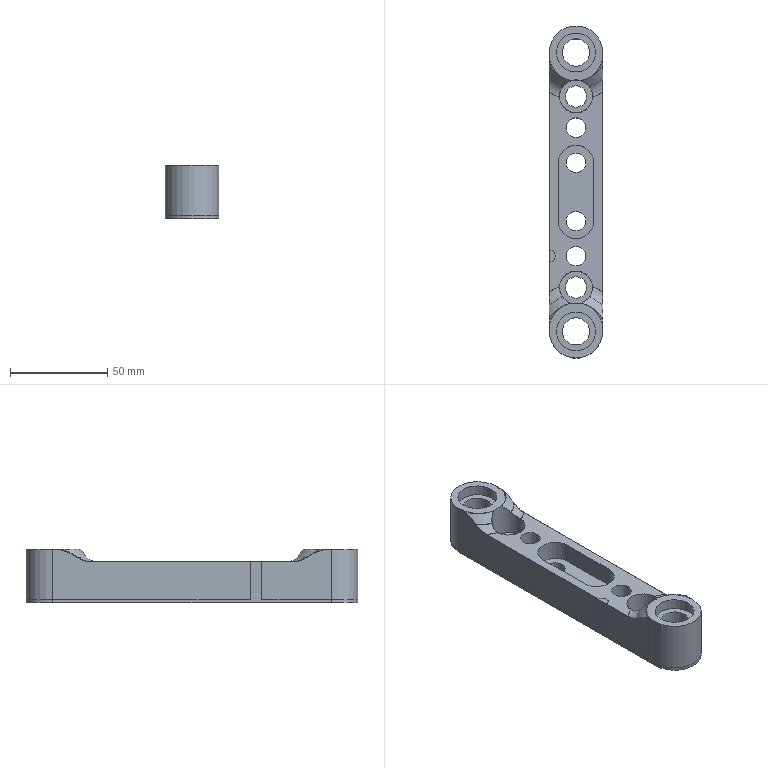NC program | NX | posted with a generic post | part box 27.4 x 170.48 x 27.5 mm
Lines 121 to 968 of 1859:
(PLANAR_MILL_12 , TOOL : D8开粗)
N204 T06 M6
N206 G54
N208 G17 G0 G90 X-73.278 Y0.754 B0. C0. S3000 M3
N210 G43 Z30. H6
N212 Z1.
N214 G94 G1 X-73.462 Y0.17 Z0.989 F600.
N216 X-73.355 Y-0.656 Z0.975
N218 X-73.016 Y-1.244 Z0.963
N220 X-72.505 Y-1.671 Z0.951
N222 X-71.879 Y-1.9 Z0.94
N224 X-71.201 Z0.928
N226 X-70.575 Y-1.671 Z0.916
N228 X-70.064 Y-1.244 Z0.905
N230 X-69.725 Y-0.656 Z0.893
N232 X-69.618 Y0.17 Z0.878
N234 X-69.869 Y0.965 Z0.864
N236 X-70.431 Y1.58 Z0.849
N238 X-71.201 Y1.9 Z0.835
N240 X-71.879 Z0.823
N242 X-72.649 Y1.58 Z0.808
N244 X-73.211 Y0.965 Z0.794
N246 X-73.462 Y0.17 Z0.779
N248 X-73.355 Y-0.656 Z0.764
N250 X-73.016 Y-1.244 Z0.753
N252 X-72.505 Y-1.671 Z0.741
N254 X-71.879 Y-1.9 Z0.729
N256 X-71.201 Z0.718
N258 X-70.575 Y-1.671 Z0.706
N260 X-70.064 Y-1.244 Z0.694
N262 X-69.725 Y-0.656 Z0.682
N264 X-69.618 Y0.17 Z0.668
N266 X-69.869 Y0.965 Z0.653
N268 X-70.431 Y1.58 Z0.639
N270 X-71.201 Y1.9 Z0.624
N272 X-71.879 Z0.612
N274 X-72.649 Y1.58 Z0.598
N276 X-73.211 Y0.965 Z0.583
N278 X-73.462 Y0.17 Z0.569
N280 X-73.355 Y-0.656 Z0.554
N282 X-73.016 Y-1.244 Z0.542
N284 X-72.505 Y-1.671 Z0.531
N286 X-71.879 Y-1.9 Z0.519
N288 X-71.201 Z0.507
N290 X-70.575 Y-1.671 Z0.496
N292 X-70.064 Y-1.244 Z0.484
N294 X-69.725 Y-0.656 Z0.472
N296 X-69.618 Y0.17 Z0.458
N298 X-69.869 Y0.965 Z0.443
N300 X-70.431 Y1.58 Z0.429
N302 X-71.201 Y1.9 Z0.414
N304 X-71.879 Z0.402
N306 X-72.649 Y1.58 Z0.388
N308 X-73.211 Y0.965 Z0.373
N310 X-73.462 Y0.17 Z0.359
N312 X-73.355 Y-0.656 Z0.344
N314 X-73.016 Y-1.244 Z0.332
N316 X-72.505 Y-1.671 Z0.321
N318 X-71.879 Y-1.9 Z0.309
N320 X-71.201 Z0.297
N322 X-70.575 Y-1.671 Z0.285
N324 X-70.064 Y-1.244 Z0.274
N326 X-69.725 Y-0.656 Z0.262
N328 X-69.618 Y0.17 Z0.247
N330 X-69.869 Y0.965 Z0.233
N332 X-70.431 Y1.58 Z0.218
N334 X-71.201 Y1.9 Z0.204
N336 X-71.879 Z0.192
N338 X-72.649 Y1.58 Z0.177
N340 X-73.211 Y0.965 Z0.163
N342 X-73.462 Y0.17 Z0.148
N344 X-73.355 Y-0.656 Z0.134
N346 X-73.016 Y-1.244 Z0.122
N348 X-72.505 Y-1.671 Z0.11
N350 X-71.879 Y-1.9 Z0.099
N352 X-71.201 Z0.087
N354 X-70.575 Y-1.671 Z0.075
N356 X-70.064 Y-1.244 Z0.064
N358 X-69.725 Y-0.656 Z0.052
N360 X-69.618 Y0.17 Z0.037
N362 X-69.869 Y0.965 Z0.023
N364 X-70.431 Y1.58 Z0.008
N366 X-71.201 Y1.9 Z-0.007
N368 X-71.879 Z-0.018
N370 X-72.649 Y1.58 Z-0.033
N372 X-73.211 Y0.965 Z-0.047
N374 X-73.462 Y0.17 Z-0.062
N376 X-73.355 Y-0.656 Z-0.077
N378 X-73.016 Y-1.244 Z-0.088
N380 X-72.505 Y-1.671 Z-0.1
N382 X-71.879 Y-1.9 Z-0.112
N384 X-71.201 Z-0.123
N386 X-70.575 Y-1.671 Z-0.135
N388 X-70.064 Y-1.244 Z-0.147
N390 X-69.725 Y-0.656 Z-0.159
N392 X-69.618 Y0.17 Z-0.173
N394 X-69.869 Y0.965 Z-0.188
N396 X-70.431 Y1.58 Z-0.202
N398 X-71.201 Y1.9 Z-0.217
N400 X-71.879 Z-0.229
N402 X-72.649 Y1.58 Z-0.243
N404 X-73.211 Y0.965 Z-0.258
N406 X-73.462 Y0.17 Z-0.272
N408 X-73.355 Y-0.656 Z-0.287
N410 X-73.016 Y-1.244 Z-0.299
N412 X-72.505 Y-1.671 Z-0.31
N414 X-71.879 Y-1.9 Z-0.322
N416 X-71.201 Z-0.334
N418 X-70.575 Y-1.671 Z-0.345
N420 X-70.064 Y-1.244 Z-0.357
N422 X-69.725 Y-0.656 Z-0.369
N424 X-69.618 Y0.17 Z-0.383
N426 X-69.869 Y0.965 Z-0.398
N428 X-70.431 Y1.58 Z-0.413
N430 X-71.201 Y1.9 Z-0.427
N432 X-71.879 Z-0.439
N434 X-72.649 Y1.58 Z-0.453
N436 X-73.211 Y0.965 Z-0.468
N438 X-73.462 Y0.17 Z-0.483
N440 X-73.355 Y-0.656 Z-0.497
N442 X-73.016 Y-1.244 Z-0.509
N444 X-72.505 Y-1.671 Z-0.521
N446 X-71.879 Y-1.9 Z-0.532
N448 X-71.201 Z-0.544
N450 X-70.575 Y-1.671 Z-0.556
N452 X-70.064 Y-1.244 Z-0.567
N454 X-69.725 Y-0.656 Z-0.579
N456 X-69.618 Y0.17 Z-0.594
N458 X-69.869 Y0.965 Z-0.608
N460 X-70.431 Y1.58 Z-0.623
N462 X-71.201 Y1.9 Z-0.637
N464 X-71.879 Z-0.649
N466 X-72.649 Y1.58 Z-0.664
N468 X-73.211 Y0.965 Z-0.678
N470 X-73.462 Y0.17 Z-0.693
N472 X-73.355 Y-0.656 Z-0.707
N474 X-73.016 Y-1.244 Z-0.719
N476 X-72.505 Y-1.671 Z-0.731
N478 X-71.879 Y-1.9 Z-0.742
N480 X-71.201 Z-0.754
N482 X-70.575 Y-1.671 Z-0.766
N484 X-70.064 Y-1.244 Z-0.778
N486 X-69.725 Y-0.656 Z-0.789
N488 X-69.618 Y0.17 Z-0.804
N490 X-69.869 Y0.965 Z-0.818
N492 X-70.431 Y1.58 Z-0.833
N494 X-71.201 Y1.9 Z-0.848
N496 X-71.879 Z-0.859
N498 X-72.649 Y1.58 Z-0.874
N500 X-73.211 Y0.965 Z-0.889
N502 X-73.462 Y0.17 Z-0.903
N504 X-73.355 Y-0.656 Z-0.918
N506 X-73.016 Y-1.244 Z-0.929
N508 X-72.505 Y-1.671 Z-0.941
N510 X-71.879 Y-1.9 Z-0.953
N512 X-71.201 Z-0.965
N514 X-70.575 Y-1.671 Z-0.976
N516 X-70.064 Y-1.244 Z-0.988
N518 X-69.725 Y-0.656 Z-1.
N520 X-69.618 Y0.17 Z-1.014
N522 X-69.869 Y0.965 Z-1.029
N524 X-70.431 Y1.58 Z-1.043
N526 X-71.201 Y1.9 Z-1.058
N528 X-71.879 Z-1.07
N530 X-72.649 Y1.58 Z-1.084
N532 X-73.211 Y0.965 Z-1.099
N534 X-73.462 Y0.17 Z-1.113
N536 X-73.355 Y-0.656 Z-1.128
N538 X-73.016 Y-1.244 Z-1.14
N540 X-72.505 Y-1.671 Z-1.151
N542 X-71.879 Y-1.9 Z-1.163
N544 X-71.201 Z-1.175
N546 X-70.575 Y-1.671 Z-1.186
N548 X-70.064 Y-1.244 Z-1.198
N550 X-69.725 Y-0.656 Z-1.21
N552 X-69.618 Y0.17 Z-1.224
N554 X-69.869 Y0.965 Z-1.239
N556 X-70.431 Y1.58 Z-1.254
N558 X-71.201 Y1.9 Z-1.268
N560 X-71.879 Z-1.28
N562 X-72.649 Y1.58 Z-1.294
N564 X-73.211 Y0.965 Z-1.309
N566 X-73.462 Y0.17 Z-1.324
N568 X-73.355 Y-0.656 Z-1.338
N570 X-73.016 Y-1.244 Z-1.35
N572 X-72.505 Y-1.671 Z-1.362
N574 X-71.879 Y-1.9 Z-1.373
N576 X-71.201 Z-1.385
N578 X-70.575 Y-1.671 Z-1.397
N580 X-70.064 Y-1.244 Z-1.408
N582 X-69.725 Y-0.656 Z-1.42
N584 X-69.618 Y0.17 Z-1.435
N586 X-69.869 Y0.965 Z-1.449
N588 X-70.431 Y1.58 Z-1.464
N590 X-71.201 Y1.9 Z-1.478
N592 X-71.879 Z-1.49
N594 X-72.649 Y1.58 Z-1.505
N596 X-73.211 Y0.965 Z-1.519
N598 X-73.462 Y0.17 Z-1.534
N600 X-73.355 Y-0.656 Z-1.548
N602 X-73.016 Y-1.244 Z-1.56
N604 X-72.505 Y-1.671 Z-1.572
N606 X-71.879 Y-1.9 Z-1.584
N608 X-71.201 Z-1.595
N610 X-70.575 Y-1.671 Z-1.607
N612 X-70.064 Y-1.244 Z-1.619
N614 X-69.725 Y-0.656 Z-1.63
N616 X-69.618 Y0.17 Z-1.645
N618 X-69.869 Y0.965 Z-1.66
N620 X-70.431 Y1.58 Z-1.674
N622 X-71.201 Y1.9 Z-1.689
N624 X-71.879 Z-1.7
N626 X-72.649 Y1.58 Z-1.715
N628 X-73.211 Y0.965 Z-1.73
N630 X-73.462 Y0.17 Z-1.744
N632 X-73.355 Y-0.656 Z-1.759
N634 X-73.016 Y-1.244 Z-1.771
N636 X-72.505 Y-1.671 Z-1.782
N638 X-71.879 Y-1.9 Z-1.794
N640 X-71.201 Z-1.806
N642 X-70.575 Y-1.671 Z-1.817
N644 X-70.064 Y-1.244 Z-1.829
N646 X-69.725 Y-0.656 Z-1.841
N648 X-69.618 Y0.17 Z-1.855
N650 X-69.869 Y0.965 Z-1.87
N652 X-70.431 Y1.58 Z-1.884
N654 X-71.201 Y1.9 Z-1.899
N656 X-71.879 Z-1.911
N658 X-72.649 Y1.58 Z-1.925
N660 X-73.211 Y0.965 Z-1.94
N662 X-73.462 Y0.17 Z-1.954
N664 X-73.355 Y-0.656 Z-1.969
N666 X-73.016 Y-1.244 Z-1.981
N668 X-72.505 Y-1.671 Z-1.992
N670 X-71.879 Y-1.9 Z-2.004
N672 X-71.201 Z-2.016
N674 X-70.575 Y-1.671 Z-2.028
N676 X-70.064 Y-1.244 Z-2.039
N678 X-69.725 Y-0.656 Z-2.051
N680 X-69.618 Y0.17 Z-2.066
N682 X-69.869 Y0.965 Z-2.08
N684 X-70.431 Y1.58 Z-2.095
N686 X-71.201 Y1.9 Z-2.109
N688 X-71.879 Z-2.121
N690 X-72.649 Y1.58 Z-2.136
N692 X-73.211 Y0.965 Z-2.15
N694 X-73.462 Y0.17 Z-2.165
N696 X-73.355 Y-0.656 Z-2.179
N698 X-73.016 Y-1.244 Z-2.191
N700 X-72.505 Y-1.671 Z-2.203
N702 X-71.879 Y-1.9 Z-2.214
N704 X-71.201 Z-2.226
N706 X-70.575 Y-1.671 Z-2.238
N708 X-70.064 Y-1.244 Z-2.249
N710 X-69.725 Y-0.656 Z-2.261
N712 X-69.618 Y0.17 Z-2.276
N714 X-69.869 Y0.965 Z-2.29
N716 X-70.431 Y1.58 Z-2.305
N718 X-71.201 Y1.9 Z-2.319
N720 X-71.879 Z-2.331
N722 X-72.649 Y1.58 Z-2.346
N724 X-73.211 Y0.965 Z-2.36
N726 X-73.462 Y0.17 Z-2.375
N728 X-73.355 Y-0.656 Z-2.389
N730 X-73.016 Y-1.244 Z-2.401
N732 X-72.505 Y-1.671 Z-2.413
N734 X-71.879 Y-1.9 Z-2.425
N736 X-71.201 Z-2.436
N738 X-70.575 Y-1.671 Z-2.448
N740 X-70.064 Y-1.244 Z-2.46
N742 X-69.725 Y-0.656 Z-2.472
N744 X-69.618 Y0.17 Z-2.486
N746 X-69.869 Y0.965 Z-2.501
N748 X-70.431 Y1.58 Z-2.515
N750 X-71.201 Y1.9 Z-2.53
N752 X-71.879 Z-2.542
N754 X-72.649 Y1.58 Z-2.556
N756 X-73.211 Y0.965 Z-2.571
N758 X-73.462 Y0.17 Z-2.585
N760 X-73.355 Y-0.656 Z-2.6
N762 X-73.016 Y-1.244 Z-2.612
N764 X-72.505 Y-1.671 Z-2.623
N766 X-71.879 Y-1.9 Z-2.635
N768 X-71.201 Z-2.647
N770 X-70.575 Y-1.671 Z-2.658
N772 X-70.064 Y-1.244 Z-2.67
N774 X-69.725 Y-0.656 Z-2.682
N776 X-69.618 Y0.17 Z-2.696
N778 X-69.869 Y0.965 Z-2.711
N780 X-70.431 Y1.58 Z-2.725
N782 X-71.201 Y1.9 Z-2.74
N784 X-71.879 Z-2.752
N786 X-72.649 Y1.58 Z-2.766
N788 X-73.211 Y0.965 Z-2.781
N790 X-73.462 Y0.17 Z-2.795
N792 X-73.355 Y-0.656 Z-2.81
N794 X-73.016 Y-1.244 Z-2.822
N796 X-72.505 Y-1.671 Z-2.833
N798 X-71.879 Y-1.9 Z-2.845
N800 X-71.201 Z-2.857
N802 X-70.575 Y-1.671 Z-2.869
N804 X-70.064 Y-1.244 Z-2.88
N806 X-69.725 Y-0.656 Z-2.892
N808 X-69.618 Y0.17 Z-2.907
N810 X-69.869 Y0.965 Z-2.921
N812 X-70.431 Y1.58 Z-2.936
N814 X-71.201 Y1.9 Z-2.95
N816 X-71.879 Z-2.962
N818 X-72.649 Y1.58 Z-2.977
N820 X-73.211 Y0.965 Z-2.991
N822 X-73.462 Y0.17 Z-3.006
N824 X-73.355 Y-0.656 Z-3.02
N826 X-73.016 Y-1.244 Z-3.032
N828 X-72.505 Y-1.671 Z-3.044
N830 X-71.879 Y-1.9 Z-3.055
N832 X-71.201 Z-3.067
N834 X-70.575 Y-1.671 Z-3.079
N836 X-70.064 Y-1.244 Z-3.09
N838 X-69.725 Y-0.656 Z-3.102
N840 X-69.618 Y0.17 Z-3.117
N842 X-69.869 Y0.965 Z-3.131
N844 X-70.431 Y1.58 Z-3.146
N846 X-71.201 Y1.9 Z-3.16
N848 X-71.879 Z-3.172
N850 X-72.649 Y1.58 Z-3.187
N852 X-73.211 Y0.965 Z-3.201
N854 X-73.462 Y0.17 Z-3.216
N856 X-73.355 Y-0.656 Z-3.231
N858 X-73.016 Y-1.244 Z-3.242
N860 X-72.505 Y-1.671 Z-3.254
N862 X-71.879 Y-1.9 Z-3.266
N864 X-71.201 Z-3.277
N866 X-70.575 Y-1.671 Z-3.289
N868 X-70.064 Y-1.244 Z-3.301
N870 X-69.725 Y-0.656 Z-3.313
N872 X-69.618 Y0.17 Z-3.327
N874 X-69.869 Y0.965 Z-3.342
N876 X-70.431 Y1.58 Z-3.356
N878 X-71.201 Y1.9 Z-3.371
N880 X-71.879 Z-3.383
N882 X-72.649 Y1.58 Z-3.397
N884 X-73.211 Y0.965 Z-3.412
N886 X-73.462 Y0.17 Z-3.426
N888 X-73.355 Y-0.656 Z-3.441
N890 X-73.016 Y-1.244 Z-3.453
N892 X-72.505 Y-1.671 Z-3.464
N894 X-71.879 Y-1.9 Z-3.476
N896 X-71.201 Z-3.488
N898 X-70.575 Y-1.671 Z-3.499
N900 X-70.064 Y-1.244 Z-3.511
N902 X-69.725 Y-0.656 Z-3.523
N904 X-69.618 Y0.17 Z-3.537
N906 X-69.869 Y0.965 Z-3.552
N908 X-70.431 Y1.58 Z-3.566
N910 X-71.201 Y1.9 Z-3.581
N912 X-71.879 Z-3.593
N914 X-72.649 Y1.58 Z-3.607
N916 X-73.211 Y0.965 Z-3.622
N918 X-73.462 Y0.17 Z-3.637
N920 X-73.355 Y-0.656 Z-3.651
N922 X-73.016 Y-1.244 Z-3.663
N924 X-72.505 Y-1.671 Z-3.675
N926 X-71.879 Y-1.9 Z-3.686
N928 X-71.201 Z-3.698
N930 X-70.575 Y-1.671 Z-3.71
N932 X-70.064 Y-1.244 Z-3.721
N934 X-69.725 Y-0.656 Z-3.733
N936 X-69.618 Y0.17 Z-3.748
N938 X-69.869 Y0.965 Z-3.762
N940 X-70.431 Y1.58 Z-3.777
N942 X-71.201 Y1.9 Z-3.791
N944 X-71.879 Z-3.803
N946 X-72.649 Y1.58 Z-3.818
N948 X-73.211 Y0.965 Z-3.832
N950 X-73.462 Y0.17 Z-3.847
N952 X-73.355 Y-0.656 Z-3.861
N954 X-73.016 Y-1.244 Z-3.873
N956 X-72.505 Y-1.671 Z-3.885
N958 X-71.879 Y-1.9 Z-3.896
N960 X-71.201 Z-3.908
N962 X-70.575 Y-1.671 Z-3.92
N964 X-70.064 Y-1.244 Z-3.932
N966 X-69.725 Y-0.656 Z-3.943
N968 X-69.618 Y0.17 Z-3.958
N970 X-69.869 Y0.965 Z-3.972
N972 X-70.431 Y1.58 Z-3.987
N974 X-71.201 Y1.9 Z-4.002
N976 X-71.879 Z-4.013
N978 X-72.649 Y1.58 Z-4.028
N980 X-73.211 Y0.965 Z-4.042
N982 X-73.462 Y0.17 Z-4.057
N984 X-73.355 Y-0.656 Z-4.072
N986 X-73.016 Y-1.244 Z-4.083
N988 X-72.505 Y-1.671 Z-4.095
N990 X-71.879 Y-1.9 Z-4.107
N992 X-71.201 Z-4.119
N994 X-70.575 Y-1.671 Z-4.13
N996 X-70.064 Y-1.244 Z-4.142
N998 X-69.725 Y-0.656 Z-4.154
N1000 X-69.618 Y0.17 Z-4.168
N1002 X-69.869 Y0.965 Z-4.183
N1004 X-70.431 Y1.58 Z-4.197
N1006 X-71.201 Y1.9 Z-4.212
N1008 X-71.879 Z-4.224
N1010 X-72.649 Y1.58 Z-4.238
N1012 X-73.211 Y0.965 Z-4.253
N1014 X-73.462 Y0.17 Z-4.267
N1016 X-73.355 Y-0.656 Z-4.282
N1018 X-73.016 Y-1.244 Z-4.294
N1020 X-72.505 Y-1.671 Z-4.305
N1022 X-71.879 Y-1.9 Z-4.317
N1024 X-71.201 Z-4.329
N1026 X-70.575 Y-1.671 Z-4.34
N1028 X-70.064 Y-1.244 Z-4.352
N1030 X-69.725 Y-0.656 Z-4.364
N1032 X-69.618 Y0.17 Z-4.378
N1034 X-69.869 Y0.965 Z-4.393
N1036 X-70.431 Y1.58 Z-4.408
N1038 X-71.201 Y1.9 Z-4.422
N1040 X-71.879 Z-4.434
N1042 X-72.649 Y1.58 Z-4.448
N1044 X-73.211 Y0.965 Z-4.463
N1046 X-73.462 Y0.17 Z-4.478
N1048 X-73.355 Y-0.656 Z-4.492
N1050 X-73.016 Y-1.244 Z-4.504
N1052 X-72.505 Y-1.671 Z-4.516
N1054 X-71.879 Y-1.9 Z-4.527
N1056 X-71.201 Z-4.539
N1058 X-70.575 Y-1.671 Z-4.551
N1060 X-70.064 Y-1.244 Z-4.562
N1062 X-69.725 Y-0.656 Z-4.574
N1064 X-69.618 Y0.17 Z-4.589
N1066 X-69.869 Y0.965 Z-4.603
N1068 X-70.431 Y1.58 Z-4.618
N1070 X-71.201 Y1.9 Z-4.632
N1072 X-71.879 Z-4.644
N1074 X-72.649 Y1.58 Z-4.659
N1076 X-73.211 Y0.965 Z-4.673
N1078 X-73.462 Y0.17 Z-4.688
N1080 X-73.355 Y-0.656 Z-4.702
N1082 X-73.016 Y-1.244 Z-4.714
N1084 X-72.505 Y-1.671 Z-4.726
N1086 X-71.879 Y-1.9 Z-4.737
N1088 X-71.201 Z-4.749
N1090 X-70.575 Y-1.671 Z-4.761
N1092 X-70.064 Y-1.244 Z-4.773
N1094 X-69.725 Y-0.656 Z-4.784
N1096 X-69.618 Y0.17 Z-4.799
N1098 X-69.869 Y0.965 Z-4.814
N1100 X-70.431 Y1.58 Z-4.828
N1102 X-71.201 Y1.9 Z-4.843
N1104 X-71.879 Z-4.854
N1106 X-72.649 Y1.58 Z-4.869
N1108 X-73.211 Y0.965 Z-4.884
N1110 X-73.462 Y0.17 Z-4.898
N1112 X-73.355 Y-0.656 Z-4.913
N1114 X-73.016 Y-1.244 Z-4.924
N1116 X-72.505 Y-1.671 Z-4.936
N1118 X-71.879 Y-1.9 Z-4.948
N1120 X-71.201 Z-4.96
N1122 X-70.575 Y-1.671 Z-4.971
N1124 X-70.064 Y-1.244 Z-4.983
N1126 X-69.725 Y-0.656 Z-4.995
N1128 X-69.618 Y0.17 Z-5.009
N1130 X-69.869 Y0.965 Z-5.024
N1132 X-70.431 Y1.58 Z-5.038
N1134 X-71.201 Y1.9 Z-5.053
N1136 X-71.879 Z-5.065
N1138 X-72.649 Y1.58 Z-5.079
N1140 X-73.211 Y0.965 Z-5.094
N1142 X-73.462 Y0.17 Z-5.108
N1144 X-73.355 Y-0.656 Z-5.123
N1146 X-73.016 Y-1.244 Z-5.135
N1148 X-72.505 Y-1.671 Z-5.146
N1150 X-71.879 Y-1.9 Z-5.158
N1152 X-71.201 Z-5.17
N1154 X-70.575 Y-1.671 Z-5.181
N1156 X-70.064 Y-1.244 Z-5.193
N1158 X-69.725 Y-0.656 Z-5.205
N1160 X-69.618 Y0.17 Z-5.219
N1162 X-69.869 Y0.965 Z-5.234
N1164 X-70.431 Y1.58 Z-5.249
N1166 X-71.201 Y1.9 Z-5.263
N1168 X-71.879 Z-5.275
N1170 X-72.649 Y1.58 Z-5.29
N1172 X-73.211 Y0.965 Z-5.304
N1174 X-73.462 Y0.17 Z-5.319
N1176 X-73.355 Y-0.656 Z-5.333
N1178 X-73.016 Y-1.244 Z-5.345
N1180 X-72.505 Y-1.671 Z-5.357
N1182 X-71.879 Y-1.9 Z-5.368
N1184 X-71.201 Z-5.38
N1186 X-70.575 Y-1.671 Z-5.392
N1188 X-70.064 Y-1.244 Z-5.403
N1190 X-69.725 Y-0.656 Z-5.415
N1192 X-69.618 Y0.17 Z-5.43
N1194 X-69.869 Y0.965 Z-5.444
N1196 X-70.431 Y1.58 Z-5.459
N1198 X-71.201 Y1.9 Z-5.473
N1200 X-71.879 Z-5.485
N1202 X-72.649 Y1.58 Z-5.5
N1204 X-73.211 Y0.965 Z-5.514
N1206 X-73.462 Y0.17 Z-5.529
N1208 X-73.355 Y-0.656 Z-5.543
N1210 X-73.016 Y-1.244 Z-5.555
N1212 X-72.505 Y-1.671 Z-5.567
N1214 X-71.879 Y-1.9 Z-5.579
N1216 X-71.201 Z-5.59
N1218 X-70.575 Y-1.671 Z-5.602
N1220 X-70.064 Y-1.244 Z-5.614
N1222 X-69.725 Y-0.656 Z-5.625
N1224 X-69.618 Y0.17 Z-5.64
N1226 X-69.869 Y0.965 Z-5.655
N1228 X-70.431 Y1.58 Z-5.669
N1230 X-71.201 Y1.9 Z-5.684
N1232 X-71.879 Z-5.695
N1234 X-72.649 Y1.58 Z-5.71
N1236 X-73.211 Y0.965 Z-5.725
N1238 X-73.462 Y0.17 Z-5.739
N1240 X-73.355 Y-0.656 Z-5.754
N1242 X-73.016 Y-1.244 Z-5.766
N1244 X-72.505 Y-1.671 Z-5.777
N1246 X-71.879 Y-1.9 Z-5.789
N1248 X-71.201 Z-5.801
N1250 X-70.575 Y-1.671 Z-5.812
N1252 X-70.064 Y-1.244 Z-5.824
N1254 X-69.725 Y-0.656 Z-5.836
N1256 X-69.618 Y0.17 Z-5.85
N1258 X-69.869 Y0.965 Z-5.865
N1260 X-70.431 Y1.58 Z-5.879
N1262 X-71.201 Y1.9 Z-5.894
N1264 X-71.879 Z-5.906
N1266 X-72.649 Y1.58 Z-5.92
N1268 X-73.211 Y0.965 Z-5.935
N1270 X-73.462 Y0.17 Z-5.949
N1272 X-73.355 Y-0.656 Z-5.964
N1274 X-73.016 Y-1.244 Z-5.976
N1276 X-72.505 Y-1.671 Z-5.987
N1278 X-71.879 Y-1.9 Z-5.999
N1280 X-71.201 Z-6.011
N1282 X-70.575 Y-1.671 Z-6.023
N1284 X-70.064 Y-1.244 Z-6.034
N1286 X-69.725 Y-0.656 Z-6.046
N1288 X-69.618 Y0.17 Z-6.061
N1290 X-69.869 Y0.965 Z-6.075
N1292 X-70.431 Y1.58 Z-6.09
N1294 X-71.201 Y1.9 Z-6.104
N1296 X-71.879 Z-6.116
N1298 X-72.649 Y1.58 Z-6.131
N1300 X-73.211 Y0.965 Z-6.145
N1302 X-73.462 Y0.17 Z-6.16
N1304 X-73.355 Y-0.656 Z-6.174
N1306 X-73.016 Y-1.244 Z-6.186
N1308 X-72.505 Y-1.671 Z-6.198
N1310 X-71.879 Y-1.9 Z-6.209
N1312 X-71.201 Z-6.221
N1314 X-70.575 Y-1.671 Z-6.233
N1316 X-70.064 Y-1.244 Z-6.244
N1318 X-69.725 Y-0.656 Z-6.256
N1320 X-69.618 Y0.17 Z-6.271
N1322 X-69.869 Y0.965 Z-6.285
N1324 X-70.431 Y1.58 Z-6.3
N1326 X-71.201 Y1.9 Z-6.314
N1328 X-71.879 Z-6.326
N1330 X-72.649 Y1.58 Z-6.341
N1332 X-73.211 Y0.965 Z-6.355
N1334 X-73.462 Y0.17 Z-6.37
N1336 X-73.355 Y-0.656 Z-6.384
N1338 X-73.016 Y-1.244 Z-6.396
N1340 X-72.505 Y-1.671 Z-6.408
N1342 X-71.879 Y-1.9 Z-6.42
N1344 X-71.201 Z-6.431
N1346 X-70.575 Y-1.671 Z-6.443
N1348 X-70.064 Y-1.244 Z-6.455
N1350 X-69.725 Y-0.656 Z-6.467
N1352 X-69.618 Y0.17 Z-6.481
N1354 X-69.869 Y0.965 Z-6.496
N1356 X-70.431 Y1.58 Z-6.51
N1358 X-71.201 Y1.9 Z-6.525
N1360 X-71.879 Z-6.537
N1362 X-72.649 Y1.58 Z-6.551
N1364 X-73.211 Y0.965 Z-6.566
N1366 X-73.462 Y0.17 Z-6.58
N1368 X-73.355 Y-0.656 Z-6.595
N1370 X-73.016 Y-1.244 Z-6.607
N1372 X-72.505 Y-1.671 Z-6.618
N1374 X-71.879 Y-1.9 Z-6.63
N1376 X-71.201 Z-6.642
N1378 X-70.575 Y-1.671 Z-6.653
N1380 X-70.064 Y-1.244 Z-6.665
N1382 X-69.725 Y-0.656 Z-6.677
N1384 X-69.618 Y0.17 Z-6.691
N1386 X-69.869 Y0.965 Z-6.706
N1388 X-70.431 Y1.58 Z-6.72
N1390 X-71.201 Y1.9 Z-6.735
N1392 X-71.879 Z-6.747
N1394 X-72.649 Y1.58 Z-6.761
N1396 X-73.211 Y0.965 Z-6.776
N1398 X-73.462 Y0.17 Z-6.79
N1400 X-73.355 Y-0.656 Z-6.805
N1402 X-73.016 Y-1.244 Z-6.817
N1404 X-72.505 Y-1.671 Z-6.828
N1406 X-71.879 Y-1.9 Z-6.84
N1408 X-71.201 Z-6.852
N1410 X-70.575 Y-1.671 Z-6.864
N1412 X-70.064 Y-1.244 Z-6.875
N1414 X-69.725 Y-0.656 Z-6.887
N1416 X-69.618 Y0.17 Z-6.902
N1418 X-69.869 Y0.965 Z-6.916
N1420 X-70.431 Y1.58 Z-6.931
N1422 X-71.201 Y1.9 Z-6.945
N1424 X-71.879 Z-6.957
N1426 X-72.649 Y1.58 Z-6.972
N1428 X-73.211 Y0.965 Z-6.986
N1430 X-73.462 Y0.17 Z-7.001
N1432 X-73.355 Y-0.656 Z-7.015
N1434 X-73.016 Y-1.244 Z-7.027
N1436 X-72.505 Y-1.671 Z-7.039
N1438 X-71.879 Y-1.9 Z-7.05
N1440 X-71.201 Z-7.062
N1442 X-70.575 Y-1.671 Z-7.074
N1444 X-70.064 Y-1.244 Z-7.085
N1446 X-69.725 Y-0.656 Z-7.097
N1448 X-69.618 Y0.17 Z-7.112
N1450 X-69.869 Y0.965 Z-7.126
N1452 X-70.431 Y1.58 Z-7.141
N1454 X-71.201 Y1.9 Z-7.156
N1456 X-71.879 Z-7.167
N1458 X-72.649 Y1.58 Z-7.182
N1460 X-73.211 Y0.965 Z-7.196
N1462 X-73.462 Y0.17 Z-7.211
N1464 X-73.355 Y-0.656 Z-7.226
N1466 X-73.016 Y-1.244 Z-7.237
N1468 X-72.505 Y-1.671 Z-7.249
N1470 X-71.879 Y-1.9 Z-7.261
N1472 X-71.201 Z-7.272
N1474 X-70.575 Y-1.671 Z-7.284
N1476 X-70.064 Y-1.244 Z-7.296
N1478 X-69.725 Y-0.656 Z-7.308
N1480 X-69.618 Y0.17 Z-7.322
N1482 X-69.869 Y0.965 Z-7.337
N1484 X-70.431 Y1.58 Z-7.351
N1486 X-71.201 Y1.9 Z-7.366
N1488 X-71.879 Z-7.378
N1490 X-72.649 Y1.58 Z-7.392
N1492 X-73.211 Y0.965 Z-7.407
N1494 X-73.462 Y0.17 Z-7.421
N1496 X-73.355 Y-0.656 Z-7.436
N1498 X-73.016 Y-1.244 Z-7.448
N1500 X-72.505 Y-1.671 Z-7.459
N1502 X-71.879 Y-1.9 Z-7.471
N1504 X-71.201 Z-7.483
N1506 X-70.575 Y-1.671 Z-7.494
N1508 X-70.064 Y-1.244 Z-7.506
N1510 X-69.725 Y-0.656 Z-7.518
N1512 X-69.618 Y0.17 Z-7.532
N1514 X-69.869 Y0.965 Z-7.547
N1516 X-70.431 Y1.58 Z-7.561
N1518 X-71.201 Y1.9 Z-7.576
N1520 X-71.879 Z-7.588
N1522 X-72.649 Y1.58 Z-7.602
N1524 X-73.211 Y0.965 Z-7.617
N1526 X-73.462 Y0.17 Z-7.632
N1528 X-73.355 Y-0.656 Z-7.646
N1530 X-73.016 Y-1.244 Z-7.658
N1532 X-72.505 Y-1.671 Z-7.67
N1534 X-71.879 Y-1.9 Z-7.681
N1536 X-71.201 Z-7.693
N1538 X-70.575 Y-1.671 Z-7.705
N1540 X-70.064 Y-1.244 Z-7.716
N1542 X-69.725 Y-0.656 Z-7.728
N1544 X-69.618 Y0.17 Z-7.743
N1546 X-69.869 Y0.965 Z-7.757
N1548 X-70.431 Y1.58 Z-7.772
N1550 X-71.201 Y1.9 Z-7.786
N1552 X-71.879 Z-7.798
N1554 X-72.649 Y1.58 Z-7.813
N1556 X-73.211 Y0.965 Z-7.827
N1558 X-73.462 Y0.17 Z-7.842
N1560 X-73.355 Y-0.656 Z-7.856
N1562 X-73.016 Y-1.244 Z-7.868
N1564 X-72.505 Y-1.671 Z-7.88
N1566 X-71.879 Y-1.9 Z-7.891
N1568 X-71.201 Z-7.903
N1570 X-70.575 Y-1.671 Z-7.915
N1572 X-70.064 Y-1.244 Z-7.927
N1574 X-69.725 Y-0.656 Z-7.938
N1576 X-69.618 Y0.17 Z-7.953
N1578 X-69.869 Y0.965 Z-7.967
N1580 X-70.431 Y1.58 Z-7.982
N1582 X-71.201 Y1.9 Z-7.997
N1584 X-71.879 Z-8.008
N1586 X-72.649 Y1.58 Z-8.023
N1588 X-73.211 Y0.965 Z-8.038
N1590 X-73.462 Y0.17 Z-8.052
N1592 X-73.355 Y-0.656 Z-8.067
N1594 X-73.016 Y-1.244 Z-8.078
N1596 X-72.505 Y-1.671 Z-8.09
N1598 X-71.879 Y-1.9 Z-8.102
N1600 X-71.201 Z-8.114
N1602 X-70.575 Y-1.671 Z-8.125
N1604 X-70.064 Y-1.244 Z-8.137
N1606 X-69.725 Y-0.656 Z-8.149
N1608 X-69.618 Y0.17 Z-8.163
N1610 X-69.869 Y0.965 Z-8.178
N1612 X-70.431 Y1.58 Z-8.192
N1614 X-71.201 Y1.9 Z-8.207
N1616 X-71.879 Z-8.219
N1618 X-72.649 Y1.58 Z-8.233
N1620 X-73.211 Y0.965 Z-8.248
N1622 X-73.462 Y0.17 Z-8.262
N1624 X-73.355 Y-0.656 Z-8.277
N1626 X-73.016 Y-1.244 Z-8.289
N1628 X-72.505 Y-1.671 Z-8.3
N1630 X-71.879 Y-1.9 Z-8.312
N1632 X-71.201 Z-8.324
N1634 X-70.575 Y-1.671 Z-8.335
N1636 X-70.064 Y-1.244 Z-8.347
N1638 X-69.725 Y-0.656 Z-8.359
N1640 X-69.618 Y0.17 Z-8.373
N1642 X-69.869 Y0.965 Z-8.388
N1644 X-70.431 Y1.58 Z-8.403
N1646 X-71.201 Y1.9 Z-8.417
N1648 X-71.879 Z-8.429
N1650 X-72.649 Y1.58 Z-8.443
N1652 X-73.211 Y0.965 Z-8.458
N1654 X-73.462 Y0.17 Z-8.473
N1656 X-73.355 Y-0.656 Z-8.487
N1658 X-73.016 Y-1.244 Z-8.499
N1660 X-72.505 Y-1.671 Z-8.511
N1662 X-71.879 Y-1.9 Z-8.522
N1664 X-71.201 Z-8.534
N1666 X-70.575 Y-1.671 Z-8.546
N1668 X-70.064 Y-1.244 Z-8.557
N1670 X-69.725 Y-0.656 Z-8.569
N1672 X-69.618 Y0.17 Z-8.584
N1674 X-69.869 Y0.965 Z-8.598
N1676 X-70.431 Y1.58 Z-8.613
N1678 X-71.201 Y1.9 Z-8.627
N1680 X-71.879 Z-8.639
N1682 X-72.649 Y1.58 Z-8.654
N1684 X-73.211 Y0.965 Z-8.668
N1686 X-73.462 Y0.17 Z-8.683
N1688 X-73.355 Y-0.656 Z-8.697
N1690 X-73.016 Y-1.244 Z-8.709
N1692 X-72.505 Y-1.671 Z-8.721
N1694 X-71.879 Y-1.9 Z-8.732
N1696 X-71.201 Z-8.744
N1698 X-70.575 Y-1.671 Z-8.756
N1700 X-70.064 Y-1.244 Z-8.768
N1702 X-69.725 Y-0.656 Z-8.779
N1704 X-69.618 Y0.17 Z-8.794
N1706 X-69.869 Y0.965 Z-8.809
N1708 X-70.431 Y1.58 Z-8.823
N1710 X-71.201 Y1.9 Z-8.838
N1712 X-71.879 Z-8.849
N1714 X-72.649 Y1.58 Z-8.864
N1716 X-73.211 Y0.965 Z-8.879
N1718 X-73.462 Y0.17 Z-8.893
N1720 X-73.355 Y-0.656 Z-8.908
N1722 X-73.016 Y-1.244 Z-8.919
N1724 X-72.505 Y-1.671 Z-8.931
N1726 X-71.879 Y-1.9 Z-8.943
N1728 X-71.201 Z-8.955
N1730 X-70.575 Y-1.671 Z-8.966
N1732 X-70.064 Y-1.244 Z-8.978
N1734 X-69.725 Y-0.656 Z-8.99
N1736 X-69.618 Y0.17 Z-9.004
N1738 X-69.869 Y0.965 Z-9.019
N1740 X-70.431 Y1.58 Z-9.033
N1742 X-71.201 Y1.9 Z-9.048
N1744 X-71.879 Z-9.06
N1746 X-72.649 Y1.58 Z-9.074
N1748 X-73.211 Y0.965 Z-9.089
N1750 X-73.462 Y0.17 Z-9.103
N1752 X-73.355 Y-0.656 Z-9.118
N1754 X-73.016 Y-1.244 Z-9.13
N1756 X-72.505 Y-1.671 Z-9.141
N1758 X-71.879 Y-1.9 Z-9.153
N1760 X-71.201 Z-9.165
N1762 X-70.575 Y-1.671 Z-9.176
N1764 X-70.064 Y-1.244 Z-9.188
N1766 X-69.725 Y-0.656 Z-9.2
N1768 X-69.618 Y0.17 Z-9.215
N1770 X-69.869 Y0.965 Z-9.229
N1772 X-70.431 Y1.58 Z-9.244
N1774 X-71.201 Y1.9 Z-9.258
N1776 X-71.879 Z-9.27
N1778 X-72.649 Y1.58 Z-9.285
N1780 X-73.211 Y0.965 Z-9.299
N1782 X-73.462 Y0.17 Z-9.314
N1784 X-73.355 Y-0.656 Z-9.328
N1786 X-73.016 Y-1.244 Z-9.34
N1788 X-72.505 Y-1.671 Z-9.352
N1790 X-71.879 Y-1.9 Z-9.363
N1792 X-71.201 Z-9.375
N1794 X-70.575 Y-1.671 Z-9.387
N1796 X-70.064 Y-1.244 Z-9.398
N1798 X-69.725 Y-0.656 Z-9.41
N1800 X-69.618 Y0.17 Z-9.425
N1802 X-69.869 Y0.965 Z-9.439
N1804 X-70.431 Y1.58 Z-9.454
N1806 X-71.201 Y1.9 Z-9.468
N1808 X-71.879 Z-9.48
N1810 X-72.649 Y1.58 Z-9.495
N1812 X-73.211 Y0.965 Z-9.509
N1814 X-73.462 Y0.17 Z-9.524
N1816 X-73.355 Y-0.656 Z-9.538
N1818 X-73.016 Y-1.244 Z-9.55
N1820 X-72.505 Y-1.671 Z-9.562
N1822 X-71.879 Y-1.9 Z-9.574
N1824 X-71.201 Z-9.585
N1826 X-70.575 Y-1.671 Z-9.597
N1828 X-70.064 Y-1.244 Z-9.609
N1830 X-69.725 Y-0.656 Z-9.62
N1832 X-69.618 Y0.17 Z-9.635
N1834 X-69.869 Y0.965 Z-9.65
N1836 X-70.431 Y1.58 Z-9.664
N1838 X-71.201 Y1.9 Z-9.679
N1840 X-71.879 Z-9.691
N1842 X-72.649 Y1.58 Z-9.705
N1844 X-73.211 Y0.965 Z-9.72
N1846 X-73.462 Y0.17 Z-9.734
N1848 X-73.355 Y-0.656 Z-9.749
N1850 X-73.016 Y-1.244 Z-9.761
N1852 X-72.505 Y-1.671 Z-9.772
N1854 X-71.879 Y-1.9 Z-9.784
N1856 X-71.201 Z-9.796
N1858 X-70.575 Y-1.671 Z-9.807
N1860 X-70.064 Y-1.244 Z-9.819
N1862 X-69.725 Y-0.656 Z-9.831
N1864 X-69.618 Y0.17 Z-9.845
N1866 X-69.869 Y0.965 Z-9.86
N1868 X-70.431 Y1.58 Z-9.874
N1870 X-71.201 Y1.9 Z-9.889
N1872 X-71.879 Z-9.901
N1874 X-72.649 Y1.58 Z-9.915
N1876 X-73.211 Y0.965 Z-9.93
N1878 X-73.462 Y0.17 Z-9.944
N1880 X-73.355 Y-0.656 Z-9.959
N1882 X-73.016 Y-1.244 Z-9.971
N1884 X-72.505 Y-1.671 Z-9.982
N1886 X-71.879 Y-1.9 Z-9.994
N1888 X-71.54 Z-10.
N1890 G3 X-69.64 Y0. R1.9
N1892 X-71.54 Y-1.9 R-1.9